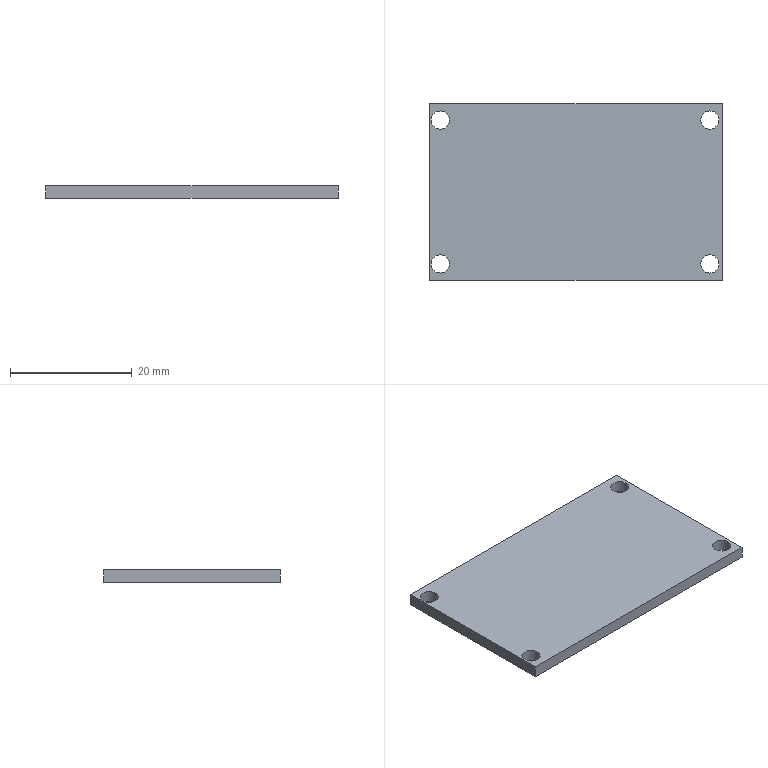Part | STEP file | Wytnij-wyci_gni_cie8[2] | 1 solid | 10 faces | box 48 x 29 x 2 mm | volume 2727 mm3 | plane 6 | cylinder 4 | commonest cylinder face diameters 3 x4
STEP:
#1=CARTESIAN_POINT('',(0.,0.,0.));
#2=DIRECTION('',(0.,0.,1.));
#3=DIRECTION('',(1.,0.,0.));
#4=AXIS2_PLACEMENT_3D('',#1,#2,#3);
#5=CARTESIAN_POINT('',(-121.918,101.438,-134.798));
#6=VERTEX_POINT('',#5);
#7=CARTESIAN_POINT('',(-121.918,99.938,-134.798));
#8=DIRECTION('',(0.,0.,1.));
#9=DIRECTION('',(0.,1.,0.));
#10=AXIS2_PLACEMENT_3D('',#7,#8,#9);
#11=CIRCLE('',#10,1.5);
#12=CARTESIAN_POINT('',(-121.918,99.938,-134.798));
#13=DIRECTION('',(0.,0.,1.));
#14=DIRECTION('',(0.,1.,0.));
#15=AXIS2_PLACEMENT_3D('',#12,#13,#14);
#16=CYLINDRICAL_SURFACE('',#15,1.5);
#17=CARTESIAN_POINT('',(0.,0.));
#18=DIRECTION('',(1.,0.));
#19=VECTOR('',#18,1.);
#20=LINE('',#17,#19);
#21=(GEOMETRIC_REPRESENTATION_CONTEXT(2)PARAMETRIC_REPRESENTATION_CONTEXT()REPRESENTATION_CONTEXT('',''));
#22=DEFINITIONAL_REPRESENTATION('',(#20),#21);
#23=PCURVE('',#16,#22);
#24=CARTESIAN_POINT('',(-99.682,88.138,-134.798));
#25=DIRECTION('',(0.,0.,-1.));
#26=DIRECTION('',(0.,-1.,0.));
#27=AXIS2_PLACEMENT_3D('',#24,#25,#26);
#28=PLANE('',#27);
#29=CARTESIAN_POINT('',(-13.3,22.237));
#30=CARTESIAN_POINT('',(-13.3,24.835));
#31=CARTESIAN_POINT('',(-11.05,23.536));
#32=CARTESIAN_POINT('',(-8.8,22.237));
#33=CARTESIAN_POINT('',(-11.05,20.938));
#34=CARTESIAN_POINT('',(-13.3,19.638));
#35=CARTESIAN_POINT('',(-13.3,22.237));
#36=(BOUNDED_CURVE()B_SPLINE_CURVE(2,(#29,#30,#31,#32,#33,#34,#35),.UNSPECIFIED.,.T.,.F.)B_SPLINE_CURVE_WITH_KNOTS((1,2,2,2,2,1),(-2.094,0.,2.094,4.189,6.283,8.378),.UNSPECIFIED.)CURVE()GEOMETRIC_REPRESENTATION_ITEM()RATIONAL_B_SPLINE_CURVE((1.,0.5,1.,0.5,1.,0.5,1.))REPRESENTATION_ITEM(''));
#37=(GEOMETRIC_REPRESENTATION_CONTEXT(2)PARAMETRIC_REPRESENTATION_CONTEXT()REPRESENTATION_CONTEXT('',''));
#38=DEFINITIONAL_REPRESENTATION('',(#36),#37);
#39=PCURVE('',#28,#38);
#40=SURFACE_CURVE('',#11,(#23,#39),.PCURVE_S1.);
#41=EDGE_CURVE('',#6,#6,#40,.T.);
#42=ORIENTED_EDGE('',*,*,#41,.T.);
#43=CARTESIAN_POINT('',(-121.918,101.438,-132.798));
#44=VERTEX_POINT('',#43);
#45=CARTESIAN_POINT('',(-121.918,101.438,-132.798));
#46=DIRECTION('',(0.,0.,-1.));
#47=VECTOR('',#46,1.);
#48=LINE('',#45,#47);
#49=CARTESIAN_POINT('',(6.283,2.));
#50=DIRECTION('',(0.,-1.));
#51=VECTOR('',#50,1.);
#52=LINE('',#49,#51);
#53=(GEOMETRIC_REPRESENTATION_CONTEXT(2)PARAMETRIC_REPRESENTATION_CONTEXT()REPRESENTATION_CONTEXT('',''));
#54=DEFINITIONAL_REPRESENTATION('',(#52),#53);
#55=PCURVE('',#16,#54);
#56=CARTESIAN_POINT('',(0.,2.));
#57=DIRECTION('',(0.,-1.));
#58=VECTOR('',#57,1.);
#59=LINE('',#56,#58);
#60=(GEOMETRIC_REPRESENTATION_CONTEXT(2)PARAMETRIC_REPRESENTATION_CONTEXT()REPRESENTATION_CONTEXT('',''));
#61=DEFINITIONAL_REPRESENTATION('',(#59),#60);
#62=PCURVE('',#16,#61);
#63=SEAM_CURVE('',#48,(#55,#62),.PCURVE_S1.);
#64=EDGE_CURVE('',#44,#6,#63,.T.);
#65=ORIENTED_EDGE('',*,*,#64,.F.);
#66=CARTESIAN_POINT('',(-121.918,99.938,-132.798));
#67=DIRECTION('',(0.,0.,-1.));
#68=DIRECTION('',(0.,1.,0.));
#69=AXIS2_PLACEMENT_3D('',#66,#67,#68);
#70=CIRCLE('',#69,1.5);
#71=CARTESIAN_POINT('',(6.283,2.));
#72=DIRECTION('',(-1.,0.));
#73=VECTOR('',#72,1.);
#74=LINE('',#71,#73);
#75=(GEOMETRIC_REPRESENTATION_CONTEXT(2)PARAMETRIC_REPRESENTATION_CONTEXT()REPRESENTATION_CONTEXT('',''));
#76=DEFINITIONAL_REPRESENTATION('',(#74),#75);
#77=PCURVE('',#16,#76);
#78=CARTESIAN_POINT('',(-99.682,88.138,-132.798));
#79=DIRECTION('',(0.,0.,-1.));
#80=DIRECTION('',(0.,-1.,0.));
#81=AXIS2_PLACEMENT_3D('',#78,#79,#80);
#82=PLANE('',#81);
#83=CARTESIAN_POINT('',(-11.8,22.237));
#84=DIRECTION('',(-1.,0.));
#85=AXIS2_PLACEMENT_2D('',#83,#84);
#86=CIRCLE('',#85,1.5);
#87=(GEOMETRIC_REPRESENTATION_CONTEXT(2)PARAMETRIC_REPRESENTATION_CONTEXT()REPRESENTATION_CONTEXT('',''));
#88=DEFINITIONAL_REPRESENTATION('',(#86),#87);
#89=PCURVE('',#82,#88);
#90=SURFACE_CURVE('',#70,(#77,#89),.PCURVE_S1.);
#91=EDGE_CURVE('',#44,#44,#90,.T.);
#92=ORIENTED_EDGE('',*,*,#91,.T.);
#93=ORIENTED_EDGE('',*,*,#64,.T.);
#94=EDGE_LOOP('',(#42,#65,#92,#93));
#95=FACE_BOUND('',#94,.F.);
#96=ADVANCED_FACE('',(#95),#16,.F.);
#97=CARTESIAN_POINT('',(-77.728,101.438,-134.798));
#98=VERTEX_POINT('',#97);
#99=CARTESIAN_POINT('',(-77.728,99.938,-134.798));
#100=DIRECTION('',(0.,0.,1.));
#101=DIRECTION('',(0.,1.,0.));
#102=AXIS2_PLACEMENT_3D('',#99,#100,#101);
#103=CIRCLE('',#102,1.5);
#104=CARTESIAN_POINT('',(-77.728,99.938,-134.798));
#105=DIRECTION('',(0.,0.,1.));
#106=DIRECTION('',(0.,1.,0.));
#107=AXIS2_PLACEMENT_3D('',#104,#105,#106);
#108=CYLINDRICAL_SURFACE('',#107,1.5);
#109=CARTESIAN_POINT('',(0.,0.));
#110=DIRECTION('',(1.,0.));
#111=VECTOR('',#110,1.);
#112=LINE('',#109,#111);
#113=(GEOMETRIC_REPRESENTATION_CONTEXT(2)PARAMETRIC_REPRESENTATION_CONTEXT()REPRESENTATION_CONTEXT('',''));
#114=DEFINITIONAL_REPRESENTATION('',(#112),#113);
#115=PCURVE('',#108,#114);
#116=CARTESIAN_POINT('',(-13.3,-21.954));
#117=CARTESIAN_POINT('',(-13.3,-19.356));
#118=CARTESIAN_POINT('',(-11.05,-20.655));
#119=CARTESIAN_POINT('',(-8.8,-21.954));
#120=CARTESIAN_POINT('',(-11.05,-23.253));
#121=CARTESIAN_POINT('',(-13.3,-24.552));
#122=CARTESIAN_POINT('',(-13.3,-21.954));
#123=(BOUNDED_CURVE()B_SPLINE_CURVE(2,(#116,#117,#118,#119,#120,#121,#122),.UNSPECIFIED.,.T.,.F.)B_SPLINE_CURVE_WITH_KNOTS((1,2,2,2,2,1),(-2.094,0.,2.094,4.189,6.283,8.378),.UNSPECIFIED.)CURVE()GEOMETRIC_REPRESENTATION_ITEM()RATIONAL_B_SPLINE_CURVE((1.,0.5,1.,0.5,1.,0.5,1.))REPRESENTATION_ITEM(''));
#124=(GEOMETRIC_REPRESENTATION_CONTEXT(2)PARAMETRIC_REPRESENTATION_CONTEXT()REPRESENTATION_CONTEXT('',''));
#125=DEFINITIONAL_REPRESENTATION('',(#123),#124);
#126=PCURVE('',#28,#125);
#127=SURFACE_CURVE('',#103,(#115,#126),.PCURVE_S1.);
#128=EDGE_CURVE('',#98,#98,#127,.T.);
#129=ORIENTED_EDGE('',*,*,#128,.T.);
#130=CARTESIAN_POINT('',(-77.728,101.438,-132.798));
#131=VERTEX_POINT('',#130);
#132=CARTESIAN_POINT('',(-77.728,101.438,-132.798));
#133=DIRECTION('',(0.,0.,-1.));
#134=VECTOR('',#133,1.);
#135=LINE('',#132,#134);
#136=CARTESIAN_POINT('',(6.283,2.));
#137=DIRECTION('',(0.,-1.));
#138=VECTOR('',#137,1.);
#139=LINE('',#136,#138);
#140=(GEOMETRIC_REPRESENTATION_CONTEXT(2)PARAMETRIC_REPRESENTATION_CONTEXT()REPRESENTATION_CONTEXT('',''));
#141=DEFINITIONAL_REPRESENTATION('',(#139),#140);
#142=PCURVE('',#108,#141);
#143=CARTESIAN_POINT('',(0.,2.));
#144=DIRECTION('',(0.,-1.));
#145=VECTOR('',#144,1.);
#146=LINE('',#143,#145);
#147=(GEOMETRIC_REPRESENTATION_CONTEXT(2)PARAMETRIC_REPRESENTATION_CONTEXT()REPRESENTATION_CONTEXT('',''));
#148=DEFINITIONAL_REPRESENTATION('',(#146),#147);
#149=PCURVE('',#108,#148);
#150=SEAM_CURVE('',#135,(#142,#149),.PCURVE_S1.);
#151=EDGE_CURVE('',#131,#98,#150,.T.);
#152=ORIENTED_EDGE('',*,*,#151,.F.);
#153=CARTESIAN_POINT('',(-77.728,99.938,-132.798));
#154=DIRECTION('',(0.,0.,-1.));
#155=DIRECTION('',(0.,1.,0.));
#156=AXIS2_PLACEMENT_3D('',#153,#154,#155);
#157=CIRCLE('',#156,1.5);
#158=CARTESIAN_POINT('',(6.283,2.));
#159=DIRECTION('',(-1.,0.));
#160=VECTOR('',#159,1.);
#161=LINE('',#158,#160);
#162=(GEOMETRIC_REPRESENTATION_CONTEXT(2)PARAMETRIC_REPRESENTATION_CONTEXT()REPRESENTATION_CONTEXT('',''));
#163=DEFINITIONAL_REPRESENTATION('',(#161),#162);
#164=PCURVE('',#108,#163);
#165=CARTESIAN_POINT('',(-11.8,-21.954));
#166=DIRECTION('',(-1.,0.));
#167=AXIS2_PLACEMENT_2D('',#165,#166);
#168=CIRCLE('',#167,1.5);
#169=(GEOMETRIC_REPRESENTATION_CONTEXT(2)PARAMETRIC_REPRESENTATION_CONTEXT()REPRESENTATION_CONTEXT('',''));
#170=DEFINITIONAL_REPRESENTATION('',(#168),#169);
#171=PCURVE('',#82,#170);
#172=SURFACE_CURVE('',#157,(#164,#171),.PCURVE_S1.);
#173=EDGE_CURVE('',#131,#131,#172,.T.);
#174=ORIENTED_EDGE('',*,*,#173,.T.);
#175=ORIENTED_EDGE('',*,*,#151,.T.);
#176=EDGE_LOOP('',(#129,#152,#174,#175));
#177=FACE_BOUND('',#176,.F.);
#178=ADVANCED_FACE('',(#177),#108,.F.);
#179=CARTESIAN_POINT('',(-77.728,77.838,-134.798));
#180=VERTEX_POINT('',#179);
#181=CARTESIAN_POINT('',(-77.728,76.338,-134.798));
#182=DIRECTION('',(0.,0.,1.));
#183=DIRECTION('',(0.,1.,0.));
#184=AXIS2_PLACEMENT_3D('',#181,#182,#183);
#185=CIRCLE('',#184,1.5);
#186=CARTESIAN_POINT('',(-77.728,76.338,-134.798));
#187=DIRECTION('',(0.,0.,1.));
#188=DIRECTION('',(0.,1.,0.));
#189=AXIS2_PLACEMENT_3D('',#186,#187,#188);
#190=CYLINDRICAL_SURFACE('',#189,1.5);
#191=CARTESIAN_POINT('',(0.,0.));
#192=DIRECTION('',(1.,0.));
#193=VECTOR('',#192,1.);
#194=LINE('',#191,#193);
#195=(GEOMETRIC_REPRESENTATION_CONTEXT(2)PARAMETRIC_REPRESENTATION_CONTEXT()REPRESENTATION_CONTEXT('',''));
#196=DEFINITIONAL_REPRESENTATION('',(#194),#195);
#197=PCURVE('',#190,#196);
#198=CARTESIAN_POINT('',(10.3,-21.954));
#199=CARTESIAN_POINT('',(10.3,-19.356));
#200=CARTESIAN_POINT('',(12.55,-20.655));
#201=CARTESIAN_POINT('',(14.8,-21.954));
#202=CARTESIAN_POINT('',(12.55,-23.253));
#203=CARTESIAN_POINT('',(10.3,-24.552));
#204=CARTESIAN_POINT('',(10.3,-21.954));
#205=(BOUNDED_CURVE()B_SPLINE_CURVE(2,(#198,#199,#200,#201,#202,#203,#204),.UNSPECIFIED.,.T.,.F.)B_SPLINE_CURVE_WITH_KNOTS((1,2,2,2,2,1),(-2.094,0.,2.094,4.189,6.283,8.378),.UNSPECIFIED.)CURVE()GEOMETRIC_REPRESENTATION_ITEM()RATIONAL_B_SPLINE_CURVE((1.,0.5,1.,0.5,1.,0.5,1.))REPRESENTATION_ITEM(''));
#206=(GEOMETRIC_REPRESENTATION_CONTEXT(2)PARAMETRIC_REPRESENTATION_CONTEXT()REPRESENTATION_CONTEXT('',''));
#207=DEFINITIONAL_REPRESENTATION('',(#205),#206);
#208=PCURVE('',#28,#207);
#209=SURFACE_CURVE('',#185,(#197,#208),.PCURVE_S1.);
#210=EDGE_CURVE('',#180,#180,#209,.T.);
#211=ORIENTED_EDGE('',*,*,#210,.T.);
#212=CARTESIAN_POINT('',(-77.728,77.838,-132.798));
#213=VERTEX_POINT('',#212);
#214=CARTESIAN_POINT('',(-77.728,77.838,-132.798));
#215=DIRECTION('',(0.,0.,-1.));
#216=VECTOR('',#215,1.);
#217=LINE('',#214,#216);
#218=CARTESIAN_POINT('',(6.283,2.));
#219=DIRECTION('',(0.,-1.));
#220=VECTOR('',#219,1.);
#221=LINE('',#218,#220);
#222=(GEOMETRIC_REPRESENTATION_CONTEXT(2)PARAMETRIC_REPRESENTATION_CONTEXT()REPRESENTATION_CONTEXT('',''));
#223=DEFINITIONAL_REPRESENTATION('',(#221),#222);
#224=PCURVE('',#190,#223);
#225=CARTESIAN_POINT('',(0.,2.));
#226=DIRECTION('',(0.,-1.));
#227=VECTOR('',#226,1.);
#228=LINE('',#225,#227);
#229=(GEOMETRIC_REPRESENTATION_CONTEXT(2)PARAMETRIC_REPRESENTATION_CONTEXT()REPRESENTATION_CONTEXT('',''));
#230=DEFINITIONAL_REPRESENTATION('',(#228),#229);
#231=PCURVE('',#190,#230);
#232=SEAM_CURVE('',#217,(#224,#231),.PCURVE_S1.);
#233=EDGE_CURVE('',#213,#180,#232,.T.);
#234=ORIENTED_EDGE('',*,*,#233,.F.);
#235=CARTESIAN_POINT('',(-77.728,76.338,-132.798));
#236=DIRECTION('',(0.,0.,-1.));
#237=DIRECTION('',(0.,1.,0.));
#238=AXIS2_PLACEMENT_3D('',#235,#236,#237);
#239=CIRCLE('',#238,1.5);
#240=CARTESIAN_POINT('',(6.283,2.));
#241=DIRECTION('',(-1.,0.));
#242=VECTOR('',#241,1.);
#243=LINE('',#240,#242);
#244=(GEOMETRIC_REPRESENTATION_CONTEXT(2)PARAMETRIC_REPRESENTATION_CONTEXT()REPRESENTATION_CONTEXT('',''));
#245=DEFINITIONAL_REPRESENTATION('',(#243),#244);
#246=PCURVE('',#190,#245);
#247=CARTESIAN_POINT('',(11.8,-21.954));
#248=DIRECTION('',(-1.,0.));
#249=AXIS2_PLACEMENT_2D('',#247,#248);
#250=CIRCLE('',#249,1.5);
#251=(GEOMETRIC_REPRESENTATION_CONTEXT(2)PARAMETRIC_REPRESENTATION_CONTEXT()REPRESENTATION_CONTEXT('',''));
#252=DEFINITIONAL_REPRESENTATION('',(#250),#251);
#253=PCURVE('',#82,#252);
#254=SURFACE_CURVE('',#239,(#246,#253),.PCURVE_S1.);
#255=EDGE_CURVE('',#213,#213,#254,.T.);
#256=ORIENTED_EDGE('',*,*,#255,.T.);
#257=ORIENTED_EDGE('',*,*,#233,.T.);
#258=EDGE_LOOP('',(#211,#234,#256,#257));
#259=FACE_BOUND('',#258,.F.);
#260=ADVANCED_FACE('',(#259),#190,.F.);
#261=CARTESIAN_POINT('',(-121.918,77.838,-134.798));
#262=VERTEX_POINT('',#261);
#263=CARTESIAN_POINT('',(-121.918,76.338,-134.798));
#264=DIRECTION('',(0.,0.,1.));
#265=DIRECTION('',(0.,1.,0.));
#266=AXIS2_PLACEMENT_3D('',#263,#264,#265);
#267=CIRCLE('',#266,1.5);
#268=CARTESIAN_POINT('',(-121.918,76.338,-134.798));
#269=DIRECTION('',(0.,0.,1.));
#270=DIRECTION('',(0.,1.,0.));
#271=AXIS2_PLACEMENT_3D('',#268,#269,#270);
#272=CYLINDRICAL_SURFACE('',#271,1.5);
#273=CARTESIAN_POINT('',(0.,0.));
#274=DIRECTION('',(1.,0.));
#275=VECTOR('',#274,1.);
#276=LINE('',#273,#275);
#277=(GEOMETRIC_REPRESENTATION_CONTEXT(2)PARAMETRIC_REPRESENTATION_CONTEXT()REPRESENTATION_CONTEXT('',''));
#278=DEFINITIONAL_REPRESENTATION('',(#276),#277);
#279=PCURVE('',#272,#278);
#280=CARTESIAN_POINT('',(10.3,22.237));
#281=CARTESIAN_POINT('',(10.3,24.835));
#282=CARTESIAN_POINT('',(12.55,23.536));
#283=CARTESIAN_POINT('',(14.8,22.237));
#284=CARTESIAN_POINT('',(12.55,20.938));
#285=CARTESIAN_POINT('',(10.3,19.638));
#286=CARTESIAN_POINT('',(10.3,22.237));
#287=(BOUNDED_CURVE()B_SPLINE_CURVE(2,(#280,#281,#282,#283,#284,#285,#286),.UNSPECIFIED.,.T.,.F.)B_SPLINE_CURVE_WITH_KNOTS((1,2,2,2,2,1),(-2.094,0.,2.094,4.189,6.283,8.378),.UNSPECIFIED.)CURVE()GEOMETRIC_REPRESENTATION_ITEM()RATIONAL_B_SPLINE_CURVE((1.,0.5,1.,0.5,1.,0.5,1.))REPRESENTATION_ITEM(''));
#288=(GEOMETRIC_REPRESENTATION_CONTEXT(2)PARAMETRIC_REPRESENTATION_CONTEXT()REPRESENTATION_CONTEXT('',''));
#289=DEFINITIONAL_REPRESENTATION('',(#287),#288);
#290=PCURVE('',#28,#289);
#291=SURFACE_CURVE('',#267,(#279,#290),.PCURVE_S1.);
#292=EDGE_CURVE('',#262,#262,#291,.T.);
#293=ORIENTED_EDGE('',*,*,#292,.T.);
#294=CARTESIAN_POINT('',(-121.918,77.838,-132.798));
#295=VERTEX_POINT('',#294);
#296=CARTESIAN_POINT('',(-121.918,77.838,-132.798));
#297=DIRECTION('',(0.,0.,-1.));
#298=VECTOR('',#297,1.);
#299=LINE('',#296,#298);
#300=CARTESIAN_POINT('',(6.283,2.));
#301=DIRECTION('',(0.,-1.));
#302=VECTOR('',#301,1.);
#303=LINE('',#300,#302);
#304=(GEOMETRIC_REPRESENTATION_CONTEXT(2)PARAMETRIC_REPRESENTATION_CONTEXT()REPRESENTATION_CONTEXT('',''));
#305=DEFINITIONAL_REPRESENTATION('',(#303),#304);
#306=PCURVE('',#272,#305);
#307=CARTESIAN_POINT('',(0.,2.));
#308=DIRECTION('',(0.,-1.));
#309=VECTOR('',#308,1.);
#310=LINE('',#307,#309);
#311=(GEOMETRIC_REPRESENTATION_CONTEXT(2)PARAMETRIC_REPRESENTATION_CONTEXT()REPRESENTATION_CONTEXT('',''));
#312=DEFINITIONAL_REPRESENTATION('',(#310),#311);
#313=PCURVE('',#272,#312);
#314=SEAM_CURVE('',#299,(#306,#313),.PCURVE_S1.);
#315=EDGE_CURVE('',#295,#262,#314,.T.);
#316=ORIENTED_EDGE('',*,*,#315,.F.);
#317=CARTESIAN_POINT('',(-121.918,76.338,-132.798));
#318=DIRECTION('',(0.,0.,-1.));
#319=DIRECTION('',(0.,1.,0.));
#320=AXIS2_PLACEMENT_3D('',#317,#318,#319);
#321=CIRCLE('',#320,1.5);
#322=CARTESIAN_POINT('',(6.283,2.));
#323=DIRECTION('',(-1.,0.));
#324=VECTOR('',#323,1.);
#325=LINE('',#322,#324);
#326=(GEOMETRIC_REPRESENTATION_CONTEXT(2)PARAMETRIC_REPRESENTATION_CONTEXT()REPRESENTATION_CONTEXT('',''));
#327=DEFINITIONAL_REPRESENTATION('',(#325),#326);
#328=PCURVE('',#272,#327);
#329=CARTESIAN_POINT('',(11.8,22.237));
#330=DIRECTION('',(-1.,0.));
#331=AXIS2_PLACEMENT_2D('',#329,#330);
#332=CIRCLE('',#331,1.5);
#333=(GEOMETRIC_REPRESENTATION_CONTEXT(2)PARAMETRIC_REPRESENTATION_CONTEXT()REPRESENTATION_CONTEXT('',''));
#334=DEFINITIONAL_REPRESENTATION('',(#332),#333);
#335=PCURVE('',#82,#334);
#336=SURFACE_CURVE('',#321,(#328,#335),.PCURVE_S1.);
#337=EDGE_CURVE('',#295,#295,#336,.T.);
#338=ORIENTED_EDGE('',*,*,#337,.T.);
#339=ORIENTED_EDGE('',*,*,#315,.T.);
#340=EDGE_LOOP('',(#293,#316,#338,#339));
#341=FACE_BOUND('',#340,.F.);
#342=ADVANCED_FACE('',(#341),#272,.F.);
#343=ORIENTED_EDGE('',*,*,#41,.T.);
#344=EDGE_LOOP('',(#343));
#345=FACE_BOUND('',#344,.T.);
#346=ORIENTED_EDGE('',*,*,#128,.T.);
#347=EDGE_LOOP('',(#346));
#348=FACE_BOUND('',#347,.T.);
#349=ORIENTED_EDGE('',*,*,#210,.T.);
#350=EDGE_LOOP('',(#349));
#351=FACE_BOUND('',#350,.T.);
#352=ORIENTED_EDGE('',*,*,#292,.T.);
#353=EDGE_LOOP('',(#352));
#354=FACE_BOUND('',#353,.T.);
#355=CARTESIAN_POINT('',(-123.682,73.638,-134.798));
#356=VERTEX_POINT('',#355);
#357=CARTESIAN_POINT('',(-123.682,102.638,-134.798));
#358=VERTEX_POINT('',#357);
#359=CARTESIAN_POINT('',(-123.682,73.638,-134.798));
#360=DIRECTION('',(0.,1.,0.));
#361=VECTOR('',#360,1.);
#362=LINE('',#359,#361);
#363=CARTESIAN_POINT('',(14.5,24.));
#364=DIRECTION('',(-1.,0.));
#365=VECTOR('',#364,1.);
#366=LINE('',#363,#365);
#367=(GEOMETRIC_REPRESENTATION_CONTEXT(2)PARAMETRIC_REPRESENTATION_CONTEXT()REPRESENTATION_CONTEXT('',''));
#368=DEFINITIONAL_REPRESENTATION('',(#366),#367);
#369=PCURVE('',#28,#368);
#370=CARTESIAN_POINT('',(-123.682,88.138,-133.798));
#371=DIRECTION('',(1.,0.,0.));
#372=DIRECTION('',(0.,0.,-1.));
#373=AXIS2_PLACEMENT_3D('',#370,#371,#372);
#374=PLANE('',#373);
#375=CARTESIAN_POINT('',(1.,-14.5));
#376=DIRECTION('',(0.,1.));
#377=VECTOR('',#376,1.);
#378=LINE('',#375,#377);
#379=(GEOMETRIC_REPRESENTATION_CONTEXT(2)PARAMETRIC_REPRESENTATION_CONTEXT()REPRESENTATION_CONTEXT('',''));
#380=DEFINITIONAL_REPRESENTATION('',(#378),#379);
#381=PCURVE('',#374,#380);
#382=SURFACE_CURVE('',#362,(#369,#381),.PCURVE_S1.);
#383=EDGE_CURVE('',#356,#358,#382,.T.);
#384=ORIENTED_EDGE('',*,*,#383,.T.);
#385=CARTESIAN_POINT('',(-75.682,102.638,-134.798));
#386=VERTEX_POINT('',#385);
#387=CARTESIAN_POINT('',(-123.682,102.638,-134.798));
#388=DIRECTION('',(1.,0.,0.));
#389=VECTOR('',#388,1.);
#390=LINE('',#387,#389);
#391=CARTESIAN_POINT('',(-14.5,24.));
#392=DIRECTION('',(0.,-1.));
#393=VECTOR('',#392,1.);
#394=LINE('',#391,#393);
#395=(GEOMETRIC_REPRESENTATION_CONTEXT(2)PARAMETRIC_REPRESENTATION_CONTEXT()REPRESENTATION_CONTEXT('',''));
#396=DEFINITIONAL_REPRESENTATION('',(#394),#395);
#397=PCURVE('',#28,#396);
#398=CARTESIAN_POINT('',(-99.682,102.638,-133.798));
#399=DIRECTION('',(0.,-1.,0.));
#400=DIRECTION('',(0.,0.,1.));
#401=AXIS2_PLACEMENT_3D('',#398,#399,#400);
#402=PLANE('',#401);
#403=CARTESIAN_POINT('',(-1.,24.));
#404=DIRECTION('',(0.,-1.));
#405=VECTOR('',#404,1.);
#406=LINE('',#403,#405);
#407=(GEOMETRIC_REPRESENTATION_CONTEXT(2)PARAMETRIC_REPRESENTATION_CONTEXT()REPRESENTATION_CONTEXT('',''));
#408=DEFINITIONAL_REPRESENTATION('',(#406),#407);
#409=PCURVE('',#402,#408);
#410=SURFACE_CURVE('',#390,(#397,#409),.PCURVE_S1.);
#411=EDGE_CURVE('',#358,#386,#410,.T.);
#412=ORIENTED_EDGE('',*,*,#411,.T.);
#413=CARTESIAN_POINT('',(-75.682,73.638,-134.798));
#414=VERTEX_POINT('',#413);
#415=CARTESIAN_POINT('',(-75.682,102.638,-134.798));
#416=DIRECTION('',(0.,-1.,0.));
#417=VECTOR('',#416,1.);
#418=LINE('',#415,#417);
#419=CARTESIAN_POINT('',(-14.5,-24.));
#420=DIRECTION('',(1.,0.));
#421=VECTOR('',#420,1.);
#422=LINE('',#419,#421);
#423=(GEOMETRIC_REPRESENTATION_CONTEXT(2)PARAMETRIC_REPRESENTATION_CONTEXT()REPRESENTATION_CONTEXT('',''));
#424=DEFINITIONAL_REPRESENTATION('',(#422),#423);
#425=PCURVE('',#28,#424);
#426=CARTESIAN_POINT('',(-75.682,88.138,-133.798));
#427=DIRECTION('',(-1.,0.,0.));
#428=DIRECTION('',(0.,0.,1.));
#429=AXIS2_PLACEMENT_3D('',#426,#427,#428);
#430=PLANE('',#429);
#431=CARTESIAN_POINT('',(-1.,14.5));
#432=DIRECTION('',(0.,-1.));
#433=VECTOR('',#432,1.);
#434=LINE('',#431,#433);
#435=(GEOMETRIC_REPRESENTATION_CONTEXT(2)PARAMETRIC_REPRESENTATION_CONTEXT()REPRESENTATION_CONTEXT('',''));
#436=DEFINITIONAL_REPRESENTATION('',(#434),#435);
#437=PCURVE('',#430,#436);
#438=SURFACE_CURVE('',#418,(#425,#437),.PCURVE_S1.);
#439=EDGE_CURVE('',#386,#414,#438,.T.);
#440=ORIENTED_EDGE('',*,*,#439,.T.);
#441=CARTESIAN_POINT('',(-75.682,73.638,-134.798));
#442=DIRECTION('',(-1.,0.,0.));
#443=VECTOR('',#442,1.);
#444=LINE('',#441,#443);
#445=CARTESIAN_POINT('',(14.5,-24.));
#446=DIRECTION('',(0.,1.));
#447=VECTOR('',#446,1.);
#448=LINE('',#445,#447);
#449=(GEOMETRIC_REPRESENTATION_CONTEXT(2)PARAMETRIC_REPRESENTATION_CONTEXT()REPRESENTATION_CONTEXT('',''));
#450=DEFINITIONAL_REPRESENTATION('',(#448),#449);
#451=PCURVE('',#28,#450);
#452=CARTESIAN_POINT('',(-99.682,73.638,-133.798));
#453=DIRECTION('',(0.,1.,0.));
#454=DIRECTION('',(0.,0.,-1.));
#455=AXIS2_PLACEMENT_3D('',#452,#453,#454);
#456=PLANE('',#455);
#457=CARTESIAN_POINT('',(1.,-24.));
#458=DIRECTION('',(0.,1.));
#459=VECTOR('',#458,1.);
#460=LINE('',#457,#459);
#461=(GEOMETRIC_REPRESENTATION_CONTEXT(2)PARAMETRIC_REPRESENTATION_CONTEXT()REPRESENTATION_CONTEXT('',''));
#462=DEFINITIONAL_REPRESENTATION('',(#460),#461);
#463=PCURVE('',#456,#462);
#464=SURFACE_CURVE('',#444,(#451,#463),.PCURVE_S1.);
#465=EDGE_CURVE('',#414,#356,#464,.T.);
#466=ORIENTED_EDGE('',*,*,#465,.T.);
#467=EDGE_LOOP('',(#384,#412,#440,#466));
#468=FACE_BOUND('',#467,.T.);
#469=ADVANCED_FACE('',(#345,#348,#351,#354,#468),#28,.T.);
#470=CARTESIAN_POINT('',(-123.682,102.638,-132.798));
#471=VERTEX_POINT('',#470);
#472=CARTESIAN_POINT('',(-123.682,102.638,-132.798));
#473=DIRECTION('',(0.,0.,-1.));
#474=VECTOR('',#473,1.);
#475=LINE('',#472,#474);
#476=CARTESIAN_POINT('',(1.,24.));
#477=DIRECTION('',(-1.,0.));
#478=VECTOR('',#477,1.);
#479=LINE('',#476,#478);
#480=(GEOMETRIC_REPRESENTATION_CONTEXT(2)PARAMETRIC_REPRESENTATION_CONTEXT()REPRESENTATION_CONTEXT('',''));
#481=DEFINITIONAL_REPRESENTATION('',(#479),#480);
#482=PCURVE('',#402,#481);
#483=CARTESIAN_POINT('',(-1.,14.5));
#484=DIRECTION('',(1.,0.));
#485=VECTOR('',#484,1.);
#486=LINE('',#483,#485);
#487=(GEOMETRIC_REPRESENTATION_CONTEXT(2)PARAMETRIC_REPRESENTATION_CONTEXT()REPRESENTATION_CONTEXT('',''));
#488=DEFINITIONAL_REPRESENTATION('',(#486),#487);
#489=PCURVE('',#374,#488);
#490=SURFACE_CURVE('',#475,(#482,#489),.PCURVE_S1.);
#491=EDGE_CURVE('',#471,#358,#490,.T.);
#492=ORIENTED_EDGE('',*,*,#491,.F.);
#493=CARTESIAN_POINT('',(-75.682,102.638,-132.798));
#494=VERTEX_POINT('',#493);
#495=CARTESIAN_POINT('',(-75.682,102.638,-132.798));
#496=DIRECTION('',(-1.,0.,0.));
#497=VECTOR('',#496,1.);
#498=LINE('',#495,#497);
#499=CARTESIAN_POINT('',(1.,-24.));
#500=DIRECTION('',(0.,1.));
#501=VECTOR('',#500,1.);
#502=LINE('',#499,#501);
#503=(GEOMETRIC_REPRESENTATION_CONTEXT(2)PARAMETRIC_REPRESENTATION_CONTEXT()REPRESENTATION_CONTEXT('',''));
#504=DEFINITIONAL_REPRESENTATION('',(#502),#503);
#505=PCURVE('',#402,#504);
#506=CARTESIAN_POINT('',(-14.5,-24.));
#507=DIRECTION('',(0.,1.));
#508=VECTOR('',#507,1.);
#509=LINE('',#506,#508);
#510=(GEOMETRIC_REPRESENTATION_CONTEXT(2)PARAMETRIC_REPRESENTATION_CONTEXT()REPRESENTATION_CONTEXT('',''));
#511=DEFINITIONAL_REPRESENTATION('',(#509),#510);
#512=PCURVE('',#82,#511);
#513=SURFACE_CURVE('',#498,(#505,#512),.PCURVE_S1.);
#514=EDGE_CURVE('',#494,#471,#513,.T.);
#515=ORIENTED_EDGE('',*,*,#514,.F.);
#516=CARTESIAN_POINT('',(-75.682,102.638,-134.798));
#517=DIRECTION('',(0.,0.,1.));
#518=VECTOR('',#517,1.);
#519=LINE('',#516,#518);
#520=CARTESIAN_POINT('',(-1.,-24.));
#521=DIRECTION('',(1.,0.));
#522=VECTOR('',#521,1.);
#523=LINE('',#520,#522);
#524=(GEOMETRIC_REPRESENTATION_CONTEXT(2)PARAMETRIC_REPRESENTATION_CONTEXT()REPRESENTATION_CONTEXT('',''));
#525=DEFINITIONAL_REPRESENTATION('',(#523),#524);
#526=PCURVE('',#402,#525);
#527=CARTESIAN_POINT('',(-1.,14.5));
#528=DIRECTION('',(1.,0.));
#529=VECTOR('',#528,1.);
#530=LINE('',#527,#529);
#531=(GEOMETRIC_REPRESENTATION_CONTEXT(2)PARAMETRIC_REPRESENTATION_CONTEXT()REPRESENTATION_CONTEXT('',''));
#532=DEFINITIONAL_REPRESENTATION('',(#530),#531);
#533=PCURVE('',#430,#532);
#534=SURFACE_CURVE('',#519,(#526,#533),.PCURVE_S1.);
#535=EDGE_CURVE('',#386,#494,#534,.T.);
#536=ORIENTED_EDGE('',*,*,#535,.F.);
#537=ORIENTED_EDGE('',*,*,#411,.F.);
#538=EDGE_LOOP('',(#492,#515,#536,#537));
#539=FACE_BOUND('',#538,.T.);
#540=ADVANCED_FACE('',(#539),#402,.F.);
#541=CARTESIAN_POINT('',(-123.682,73.638,-132.798));
#542=VERTEX_POINT('',#541);
#543=CARTESIAN_POINT('',(-123.682,73.638,-132.798));
#544=DIRECTION('',(0.,0.,-1.));
#545=VECTOR('',#544,1.);
#546=LINE('',#543,#545);
#547=CARTESIAN_POINT('',(-1.,-14.5));
#548=DIRECTION('',(1.,0.));
#549=VECTOR('',#548,1.);
#550=LINE('',#547,#549);
#551=(GEOMETRIC_REPRESENTATION_CONTEXT(2)PARAMETRIC_REPRESENTATION_CONTEXT()REPRESENTATION_CONTEXT('',''));
#552=DEFINITIONAL_REPRESENTATION('',(#550),#551);
#553=PCURVE('',#374,#552);
#554=CARTESIAN_POINT('',(-1.,24.));
#555=DIRECTION('',(1.,0.));
#556=VECTOR('',#555,1.);
#557=LINE('',#554,#556);
#558=(GEOMETRIC_REPRESENTATION_CONTEXT(2)PARAMETRIC_REPRESENTATION_CONTEXT()REPRESENTATION_CONTEXT('',''));
#559=DEFINITIONAL_REPRESENTATION('',(#557),#558);
#560=PCURVE('',#456,#559);
#561=SURFACE_CURVE('',#546,(#553,#560),.PCURVE_S1.);
#562=EDGE_CURVE('',#542,#356,#561,.T.);
#563=ORIENTED_EDGE('',*,*,#562,.F.);
#564=CARTESIAN_POINT('',(-123.682,102.638,-132.798));
#565=DIRECTION('',(0.,-1.,0.));
#566=VECTOR('',#565,1.);
#567=LINE('',#564,#566);
#568=CARTESIAN_POINT('',(-1.,14.5));
#569=DIRECTION('',(0.,-1.));
#570=VECTOR('',#569,1.);
#571=LINE('',#568,#570);
#572=(GEOMETRIC_REPRESENTATION_CONTEXT(2)PARAMETRIC_REPRESENTATION_CONTEXT()REPRESENTATION_CONTEXT('',''));
#573=DEFINITIONAL_REPRESENTATION('',(#571),#572);
#574=PCURVE('',#374,#573);
#575=CARTESIAN_POINT('',(-14.5,24.));
#576=DIRECTION('',(1.,0.));
#577=VECTOR('',#576,1.);
#578=LINE('',#575,#577);
#579=(GEOMETRIC_REPRESENTATION_CONTEXT(2)PARAMETRIC_REPRESENTATION_CONTEXT()REPRESENTATION_CONTEXT('',''));
#580=DEFINITIONAL_REPRESENTATION('',(#578),#579);
#581=PCURVE('',#82,#580);
#582=SURFACE_CURVE('',#567,(#574,#581),.PCURVE_S1.);
#583=EDGE_CURVE('',#471,#542,#582,.T.);
#584=ORIENTED_EDGE('',*,*,#583,.F.);
#585=ORIENTED_EDGE('',*,*,#491,.T.);
#586=ORIENTED_EDGE('',*,*,#383,.F.);
#587=EDGE_LOOP('',(#563,#584,#585,#586));
#588=FACE_BOUND('',#587,.T.);
#589=ADVANCED_FACE('',(#588),#374,.F.);
#590=CARTESIAN_POINT('',(-75.682,73.638,-132.798));
#591=VERTEX_POINT('',#590);
#592=CARTESIAN_POINT('',(-75.682,73.638,-132.798));
#593=DIRECTION('',(0.,0.,-1.));
#594=VECTOR('',#593,1.);
#595=LINE('',#592,#594);
#596=CARTESIAN_POINT('',(-1.,-24.));
#597=DIRECTION('',(1.,0.));
#598=VECTOR('',#597,1.);
#599=LINE('',#596,#598);
#600=(GEOMETRIC_REPRESENTATION_CONTEXT(2)PARAMETRIC_REPRESENTATION_CONTEXT()REPRESENTATION_CONTEXT('',''));
#601=DEFINITIONAL_REPRESENTATION('',(#599),#600);
#602=PCURVE('',#456,#601);
#603=CARTESIAN_POINT('',(1.,-14.5));
#604=DIRECTION('',(-1.,0.));
#605=VECTOR('',#604,1.);
#606=LINE('',#603,#605);
#607=(GEOMETRIC_REPRESENTATION_CONTEXT(2)PARAMETRIC_REPRESENTATION_CONTEXT()REPRESENTATION_CONTEXT('',''));
#608=DEFINITIONAL_REPRESENTATION('',(#606),#607);
#609=PCURVE('',#430,#608);
#610=SURFACE_CURVE('',#595,(#602,#609),.PCURVE_S1.);
#611=EDGE_CURVE('',#591,#414,#610,.T.);
#612=ORIENTED_EDGE('',*,*,#611,.F.);
#613=CARTESIAN_POINT('',(-123.682,73.638,-132.798));
#614=DIRECTION('',(1.,0.,0.));
#615=VECTOR('',#614,1.);
#616=LINE('',#613,#615);
#617=CARTESIAN_POINT('',(-1.,24.));
#618=DIRECTION('',(0.,-1.));
#619=VECTOR('',#618,1.);
#620=LINE('',#617,#619);
#621=(GEOMETRIC_REPRESENTATION_CONTEXT(2)PARAMETRIC_REPRESENTATION_CONTEXT()REPRESENTATION_CONTEXT('',''));
#622=DEFINITIONAL_REPRESENTATION('',(#620),#621);
#623=PCURVE('',#456,#622);
#624=CARTESIAN_POINT('',(14.5,24.));
#625=DIRECTION('',(0.,-1.));
#626=VECTOR('',#625,1.);
#627=LINE('',#624,#626);
#628=(GEOMETRIC_REPRESENTATION_CONTEXT(2)PARAMETRIC_REPRESENTATION_CONTEXT()REPRESENTATION_CONTEXT('',''));
#629=DEFINITIONAL_REPRESENTATION('',(#627),#628);
#630=PCURVE('',#82,#629);
#631=SURFACE_CURVE('',#616,(#623,#630),.PCURVE_S1.);
#632=EDGE_CURVE('',#542,#591,#631,.T.);
#633=ORIENTED_EDGE('',*,*,#632,.F.);
#634=ORIENTED_EDGE('',*,*,#562,.T.);
#635=ORIENTED_EDGE('',*,*,#465,.F.);
#636=EDGE_LOOP('',(#612,#633,#634,#635));
#637=FACE_BOUND('',#636,.T.);
#638=ADVANCED_FACE('',(#637),#456,.F.);
#639=ORIENTED_EDGE('',*,*,#535,.T.);
#640=CARTESIAN_POINT('',(-75.682,73.638,-132.798));
#641=DIRECTION('',(0.,1.,0.));
#642=VECTOR('',#641,1.);
#643=LINE('',#640,#642);
#644=CARTESIAN_POINT('',(1.,-14.5));
#645=DIRECTION('',(0.,1.));
#646=VECTOR('',#645,1.);
#647=LINE('',#644,#646);
#648=(GEOMETRIC_REPRESENTATION_CONTEXT(2)PARAMETRIC_REPRESENTATION_CONTEXT()REPRESENTATION_CONTEXT('',''));
#649=DEFINITIONAL_REPRESENTATION('',(#647),#648);
#650=PCURVE('',#430,#649);
#651=CARTESIAN_POINT('',(14.5,-24.));
#652=DIRECTION('',(-1.,0.));
#653=VECTOR('',#652,1.);
#654=LINE('',#651,#653);
#655=(GEOMETRIC_REPRESENTATION_CONTEXT(2)PARAMETRIC_REPRESENTATION_CONTEXT()REPRESENTATION_CONTEXT('',''));
#656=DEFINITIONAL_REPRESENTATION('',(#654),#655);
#657=PCURVE('',#82,#656);
#658=SURFACE_CURVE('',#643,(#650,#657),.PCURVE_S1.);
#659=EDGE_CURVE('',#591,#494,#658,.T.);
#660=ORIENTED_EDGE('',*,*,#659,.F.);
#661=ORIENTED_EDGE('',*,*,#611,.T.);
#662=ORIENTED_EDGE('',*,*,#439,.F.);
#663=EDGE_LOOP('',(#639,#660,#661,#662));
#664=FACE_BOUND('',#663,.T.);
#665=ADVANCED_FACE('',(#664),#430,.F.);
#666=ORIENTED_EDGE('',*,*,#91,.T.);
#667=EDGE_LOOP('',(#666));
#668=FACE_BOUND('',#667,.T.);
#669=ORIENTED_EDGE('',*,*,#173,.T.);
#670=EDGE_LOOP('',(#669));
#671=FACE_BOUND('',#670,.T.);
#672=ORIENTED_EDGE('',*,*,#255,.T.);
#673=EDGE_LOOP('',(#672));
#674=FACE_BOUND('',#673,.T.);
#675=ORIENTED_EDGE('',*,*,#337,.T.);
#676=EDGE_LOOP('',(#675));
#677=FACE_BOUND('',#676,.T.);
#678=ORIENTED_EDGE('',*,*,#659,.T.);
#679=ORIENTED_EDGE('',*,*,#514,.T.);
#680=ORIENTED_EDGE('',*,*,#583,.T.);
#681=ORIENTED_EDGE('',*,*,#632,.T.);
#682=EDGE_LOOP('',(#678,#679,#680,#681));
#683=FACE_BOUND('',#682,.T.);
#684=ADVANCED_FACE('',(#668,#671,#674,#677,#683),#82,.F.);
#685=CLOSED_SHELL('',(#96,#178,#260,#342,#469,#540,#589,#638,#665,#684));
#686=MANIFOLD_SOLID_BREP('',#685);
#687=(LENGTH_UNIT()NAMED_UNIT(*)SI_UNIT(.MILLI.,.METRE.));
#688=UNCERTAINTY_MEASURE_WITH_UNIT(LENGTH_MEASURE(0.0000001),#687,'','');
#689=(NAMED_UNIT(*)PLANE_ANGLE_UNIT()SI_UNIT($,.RADIAN.));
#690=(NAMED_UNIT(*)SI_UNIT($,.STERADIAN.)SOLID_ANGLE_UNIT());
#691=(GEOMETRIC_REPRESENTATION_CONTEXT(3)GLOBAL_UNCERTAINTY_ASSIGNED_CONTEXT((#688))GLOBAL_UNIT_ASSIGNED_CONTEXT((#687,#689,#690))REPRESENTATION_CONTEXT('',''));
#692=ADVANCED_BREP_SHAPE_REPRESENTATION('',(#4,#686),#691);